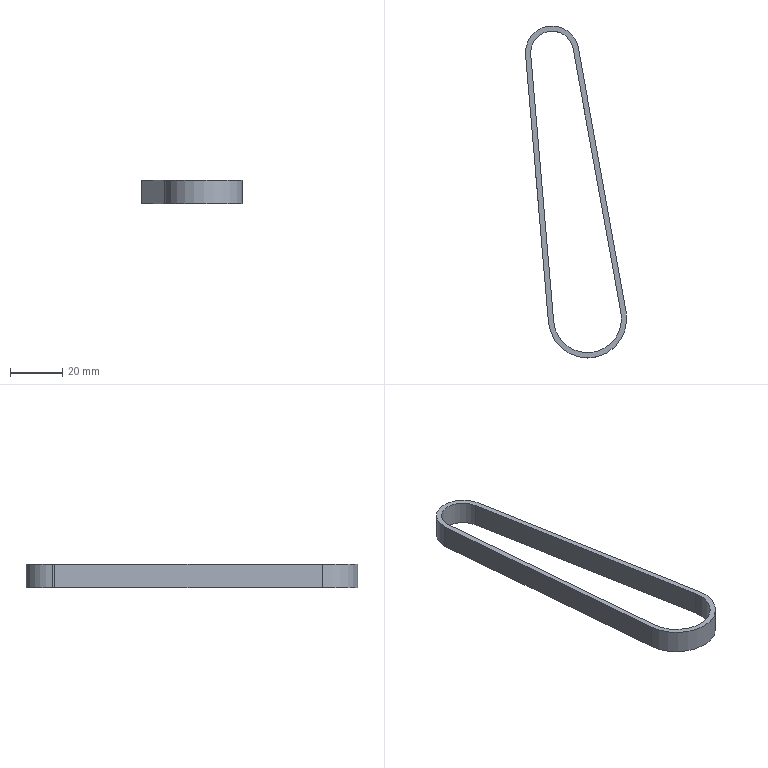Part | NX | features BREP 1 | 1 solid | 12 faces | box 38.615 x 126.615 x 9 mm | volume 4997 mm3 | plane 6 | cylinder 6 | commonest cylinder face diameters 16.34 x2 20.34 x2 25.89 x1 29.89 x1
STEP:
#1=CARTESIAN_POINT('',(26.238,-99.197,-4.5));
#2=VERTEX_POINT('',#1);
#3=CARTESIAN_POINT('',(8.04,1.454,-4.5));
#4=VERTEX_POINT('',#3);
#5=CARTESIAN_POINT('',(8.04,1.454,-4.5));
#6=DIRECTION('',(-0.1779,0.984,0.));
#7=VECTOR('',#6,1000.);
#8=LINE('',#5,#7);
#9=EDGE_CURVE('',#2,#4,#8,.T.);
#10=ORIENTED_EDGE('',*,*,#9,.F.);
#11=CARTESIAN_POINT('',(26.238,-99.197,4.5));
#12=VERTEX_POINT('',#11);
#13=CARTESIAN_POINT('',(26.238,-99.197,4.5));
#14=DIRECTION('',(0.,0.,-1.));
#15=VECTOR('',#14,1000.);
#16=LINE('',#13,#15);
#17=EDGE_CURVE('',#12,#2,#16,.T.);
#18=ORIENTED_EDGE('',*,*,#17,.F.);
#19=CARTESIAN_POINT('',(8.04,1.454,4.5));
#20=VERTEX_POINT('',#19);
#21=CARTESIAN_POINT('',(8.04,1.454,4.5));
#22=DIRECTION('',(-0.1779,0.984,0.));
#23=VECTOR('',#22,1000.);
#24=LINE('',#21,#23);
#25=EDGE_CURVE('',#12,#20,#24,.T.);
#26=ORIENTED_EDGE('',*,*,#25,.T.);
#27=CARTESIAN_POINT('',(8.04,1.454,4.5));
#28=DIRECTION('',(0.,0.,-1.));
#29=VECTOR('',#28,1000.);
#30=LINE('',#27,#29);
#31=EDGE_CURVE('',#20,#4,#30,.T.);
#32=ORIENTED_EDGE('',*,*,#31,.T.);
#33=EDGE_LOOP('',(#10,#18,#26,#32));
#34=FACE_BOUND('',#33,.T.);
#35=CARTESIAN_POINT('',(8.04,1.454,4.5));
#36=DIRECTION('',(-0.984,-0.1779,0.));
#37=DIRECTION('',(0.1779,-0.984,0.));
#38=AXIS2_PLACEMENT_3D('',#35,#36,#37);
#39=PLANE('',#38);
#40=ADVANCED_FACE('',(#34),#39,.T.);
#41=CARTESIAN_POINT('',(0.6024,-102.606,-4.5));
#42=VERTEX_POINT('',#41);
#43=CARTESIAN_POINT('',(13.5,-101.5,-4.5));
#44=DIRECTION('',(0.,0.,1.));
#45=DIRECTION('',(-1.,0.,0.));
#46=AXIS2_PLACEMENT_3D('',#43,#44,#45);
#47=CIRCLE('',#46,12.945);
#48=EDGE_CURVE('',#42,#2,#47,.T.);
#49=ORIENTED_EDGE('',*,*,#48,.F.);
#50=CARTESIAN_POINT('',(0.6024,-102.606,4.5));
#51=VERTEX_POINT('',#50);
#52=CARTESIAN_POINT('',(0.6024,-102.606,4.5));
#53=DIRECTION('',(0.,0.,-1.));
#54=VECTOR('',#53,1000.);
#55=LINE('',#52,#54);
#56=EDGE_CURVE('',#51,#42,#55,.T.);
#57=ORIENTED_EDGE('',*,*,#56,.F.);
#58=CARTESIAN_POINT('',(13.5,-101.5,4.5));
#59=DIRECTION('',(0.,0.,1.));
#60=DIRECTION('',(-1.,0.,0.));
#61=AXIS2_PLACEMENT_3D('',#58,#59,#60);
#62=CIRCLE('',#61,12.945);
#63=EDGE_CURVE('',#51,#12,#62,.T.);
#64=ORIENTED_EDGE('',*,*,#63,.T.);
#65=ORIENTED_EDGE('',*,*,#17,.T.);
#66=EDGE_LOOP('',(#49,#57,#64,#65));
#67=FACE_BOUND('',#66,.T.);
#68=CARTESIAN_POINT('',(13.5,-101.5,4.5));
#69=DIRECTION('',(0.,0.,-1.));
#70=DIRECTION('',(-1.,0.,0.));
#71=AXIS2_PLACEMENT_3D('',#68,#69,#70);
#72=CYLINDRICAL_SURFACE('',#71,12.945);
#73=ADVANCED_FACE('',(#67),#72,.F.);
#74=CARTESIAN_POINT('',(-8.14,-0.6983,-4.5));
#75=VERTEX_POINT('',#74);
#76=CARTESIAN_POINT('',(-8.14,-0.6983,-4.5));
#77=DIRECTION('',(0.08547,-0.9963,0.));
#78=VECTOR('',#77,1000.);
#79=LINE('',#76,#78);
#80=EDGE_CURVE('',#75,#42,#79,.T.);
#81=ORIENTED_EDGE('',*,*,#80,.F.);
#82=CARTESIAN_POINT('',(-8.14,-0.6983,4.5));
#83=VERTEX_POINT('',#82);
#84=CARTESIAN_POINT('',(-8.14,-0.6983,4.5));
#85=DIRECTION('',(0.,0.,-1.));
#86=VECTOR('',#85,1000.);
#87=LINE('',#84,#86);
#88=EDGE_CURVE('',#83,#75,#87,.T.);
#89=ORIENTED_EDGE('',*,*,#88,.F.);
#90=CARTESIAN_POINT('',(-8.14,-0.6983,4.5));
#91=DIRECTION('',(0.08547,-0.9963,0.));
#92=VECTOR('',#91,1000.);
#93=LINE('',#90,#92);
#94=EDGE_CURVE('',#83,#51,#93,.T.);
#95=ORIENTED_EDGE('',*,*,#94,.T.);
#96=ORIENTED_EDGE('',*,*,#56,.T.);
#97=EDGE_LOOP('',(#81,#89,#95,#96));
#98=FACE_BOUND('',#97,.T.);
#99=CARTESIAN_POINT('',(-8.14,-0.6983,4.5));
#100=DIRECTION('',(0.9963,0.08547,0.));
#101=DIRECTION('',(-0.08547,0.9963,0.));
#102=AXIS2_PLACEMENT_3D('',#99,#100,#101);
#103=PLANE('',#102);
#104=ADVANCED_FACE('',(#98),#103,.T.);
#105=CARTESIAN_POINT('',(-8.17,0.,4.5));
#106=VERTEX_POINT('',#105);
#107=CARTESIAN_POINT('',(-8.17,0.,-4.5));
#108=VERTEX_POINT('',#107);
#109=CARTESIAN_POINT('',(-8.17,0.,4.5));
#110=DIRECTION('',(0.,0.,-1.));
#111=VECTOR('',#110,1000.);
#112=LINE('',#109,#111);
#113=EDGE_CURVE('',#106,#108,#112,.T.);
#114=ORIENTED_EDGE('',*,*,#113,.F.);
#115=CARTESIAN_POINT('',(0.,0.,4.5));
#116=DIRECTION('',(0.,0.,1.));
#117=DIRECTION('',(-1.,0.,0.));
#118=AXIS2_PLACEMENT_3D('',#115,#116,#117);
#119=CIRCLE('',#118,8.17);
#120=EDGE_CURVE('',#106,#83,#119,.T.);
#121=ORIENTED_EDGE('',*,*,#120,.T.);
#122=ORIENTED_EDGE('',*,*,#88,.T.);
#123=CARTESIAN_POINT('',(0.,0.,-4.5));
#124=DIRECTION('',(0.,0.,1.));
#125=DIRECTION('',(-1.,0.,0.));
#126=AXIS2_PLACEMENT_3D('',#123,#124,#125);
#127=CIRCLE('',#126,8.17);
#128=EDGE_CURVE('',#108,#75,#127,.T.);
#129=ORIENTED_EDGE('',*,*,#128,.F.);
#130=EDGE_LOOP('',(#114,#121,#122,#129));
#131=FACE_BOUND('',#130,.T.);
#132=CARTESIAN_POINT('',(0.,0.,4.5));
#133=DIRECTION('',(0.,0.,-1.));
#134=DIRECTION('',(-1.,0.,0.));
#135=AXIS2_PLACEMENT_3D('',#132,#133,#134);
#136=CYLINDRICAL_SURFACE('',#135,8.17);
#137=ADVANCED_FACE('',(#131),#136,.F.);
#138=CARTESIAN_POINT('',(28.207,-98.841,-4.5));
#139=VERTEX_POINT('',#138);
#140=CARTESIAN_POINT('',(10.008,1.81,-4.5));
#141=VERTEX_POINT('',#140);
#142=CARTESIAN_POINT('',(10.008,1.81,-4.5));
#143=DIRECTION('',(-0.1779,0.984,0.));
#144=VECTOR('',#143,1000.);
#145=LINE('',#142,#144);
#146=EDGE_CURVE('',#139,#141,#145,.T.);
#147=ORIENTED_EDGE('',*,*,#146,.T.);
#148=CARTESIAN_POINT('',(10.008,1.81,4.5));
#149=VERTEX_POINT('',#148);
#150=CARTESIAN_POINT('',(10.008,1.81,4.5));
#151=DIRECTION('',(0.,0.,-1.));
#152=VECTOR('',#151,1000.);
#153=LINE('',#150,#152);
#154=EDGE_CURVE('',#149,#141,#153,.T.);
#155=ORIENTED_EDGE('',*,*,#154,.F.);
#156=CARTESIAN_POINT('',(28.207,-98.841,4.5));
#157=VERTEX_POINT('',#156);
#158=CARTESIAN_POINT('',(10.008,1.81,4.5));
#159=DIRECTION('',(-0.1779,0.984,0.));
#160=VECTOR('',#159,1000.);
#161=LINE('',#158,#160);
#162=EDGE_CURVE('',#157,#149,#161,.T.);
#163=ORIENTED_EDGE('',*,*,#162,.F.);
#164=CARTESIAN_POINT('',(28.207,-98.841,4.5));
#165=DIRECTION('',(0.,0.,-1.));
#166=VECTOR('',#165,1000.);
#167=LINE('',#164,#166);
#168=EDGE_CURVE('',#157,#139,#167,.T.);
#169=ORIENTED_EDGE('',*,*,#168,.T.);
#170=EDGE_LOOP('',(#147,#155,#163,#169));
#171=FACE_BOUND('',#170,.T.);
#172=CARTESIAN_POINT('',(10.008,1.81,4.5));
#173=DIRECTION('',(-0.984,-0.1779,0.));
#174=DIRECTION('',(0.1779,-0.984,0.));
#175=AXIS2_PLACEMENT_3D('',#172,#173,#174);
#176=PLANE('',#175);
#177=ADVANCED_FACE('',(#171),#176,.F.);
#178=CARTESIAN_POINT('',(-1.39,-102.777,-4.5));
#179=VERTEX_POINT('',#178);
#180=CARTESIAN_POINT('',(13.5,-101.5,-4.5));
#181=DIRECTION('',(0.,0.,1.));
#182=DIRECTION('',(-1.,0.,0.));
#183=AXIS2_PLACEMENT_3D('',#180,#181,#182);
#184=CIRCLE('',#183,14.945);
#185=EDGE_CURVE('',#179,#139,#184,.T.);
#186=ORIENTED_EDGE('',*,*,#185,.T.);
#187=ORIENTED_EDGE('',*,*,#168,.F.);
#188=CARTESIAN_POINT('',(-1.39,-102.777,4.5));
#189=VERTEX_POINT('',#188);
#190=CARTESIAN_POINT('',(13.5,-101.5,4.5));
#191=DIRECTION('',(0.,0.,1.));
#192=DIRECTION('',(-1.,0.,0.));
#193=AXIS2_PLACEMENT_3D('',#190,#191,#192);
#194=CIRCLE('',#193,14.945);
#195=EDGE_CURVE('',#189,#157,#194,.T.);
#196=ORIENTED_EDGE('',*,*,#195,.F.);
#197=CARTESIAN_POINT('',(-1.39,-102.777,4.5));
#198=DIRECTION('',(0.,0.,-1.));
#199=VECTOR('',#198,1000.);
#200=LINE('',#197,#199);
#201=EDGE_CURVE('',#189,#179,#200,.T.);
#202=ORIENTED_EDGE('',*,*,#201,.T.);
#203=EDGE_LOOP('',(#186,#187,#196,#202));
#204=FACE_BOUND('',#203,.T.);
#205=CARTESIAN_POINT('',(13.5,-101.5,4.5));
#206=DIRECTION('',(0.,0.,-1.));
#207=DIRECTION('',(-1.,0.,0.));
#208=AXIS2_PLACEMENT_3D('',#205,#206,#207);
#209=CYLINDRICAL_SURFACE('',#208,14.945);
#210=ADVANCED_FACE('',(#204),#209,.T.);
#211=CARTESIAN_POINT('',(-10.133,-0.8693,-4.5));
#212=VERTEX_POINT('',#211);
#213=CARTESIAN_POINT('',(-10.133,-0.8693,-4.5));
#214=DIRECTION('',(0.08547,-0.9963,0.));
#215=VECTOR('',#214,1000.);
#216=LINE('',#213,#215);
#217=EDGE_CURVE('',#212,#179,#216,.T.);
#218=ORIENTED_EDGE('',*,*,#217,.T.);
#219=ORIENTED_EDGE('',*,*,#201,.F.);
#220=CARTESIAN_POINT('',(-10.133,-0.8693,4.5));
#221=VERTEX_POINT('',#220);
#222=CARTESIAN_POINT('',(-10.133,-0.8693,4.5));
#223=DIRECTION('',(0.08547,-0.9963,0.));
#224=VECTOR('',#223,1000.);
#225=LINE('',#222,#224);
#226=EDGE_CURVE('',#221,#189,#225,.T.);
#227=ORIENTED_EDGE('',*,*,#226,.F.);
#228=CARTESIAN_POINT('',(-10.133,-0.8693,4.5));
#229=DIRECTION('',(0.,0.,-1.));
#230=VECTOR('',#229,1000.);
#231=LINE('',#228,#230);
#232=EDGE_CURVE('',#221,#212,#231,.T.);
#233=ORIENTED_EDGE('',*,*,#232,.T.);
#234=EDGE_LOOP('',(#218,#219,#227,#233));
#235=FACE_BOUND('',#234,.T.);
#236=CARTESIAN_POINT('',(-10.133,-0.8693,4.5));
#237=DIRECTION('',(0.9963,0.08547,0.));
#238=DIRECTION('',(-0.08547,0.9963,0.));
#239=AXIS2_PLACEMENT_3D('',#236,#237,#238);
#240=PLANE('',#239);
#241=ADVANCED_FACE('',(#235),#240,.F.);
#242=CARTESIAN_POINT('',(-10.17,0.,4.5));
#243=VERTEX_POINT('',#242);
#244=CARTESIAN_POINT('',(-10.17,0.,-4.5));
#245=VERTEX_POINT('',#244);
#246=CARTESIAN_POINT('',(-10.17,0.,4.5));
#247=DIRECTION('',(0.,0.,-1.));
#248=VECTOR('',#247,1000.);
#249=LINE('',#246,#248);
#250=EDGE_CURVE('',#243,#245,#249,.T.);
#251=ORIENTED_EDGE('',*,*,#250,.F.);
#252=CARTESIAN_POINT('',(0.,0.,4.5));
#253=DIRECTION('',(0.,0.,1.));
#254=DIRECTION('',(-1.,0.,0.));
#255=AXIS2_PLACEMENT_3D('',#252,#253,#254);
#256=CIRCLE('',#255,10.17);
#257=EDGE_CURVE('',#149,#243,#256,.T.);
#258=ORIENTED_EDGE('',*,*,#257,.F.);
#259=ORIENTED_EDGE('',*,*,#154,.T.);
#260=CARTESIAN_POINT('',(0.,0.,-4.5));
#261=DIRECTION('',(0.,0.,1.));
#262=DIRECTION('',(-1.,0.,0.));
#263=AXIS2_PLACEMENT_3D('',#260,#261,#262);
#264=CIRCLE('',#263,10.17);
#265=EDGE_CURVE('',#141,#245,#264,.T.);
#266=ORIENTED_EDGE('',*,*,#265,.T.);
#267=EDGE_LOOP('',(#251,#258,#259,#266));
#268=FACE_BOUND('',#267,.T.);
#269=CARTESIAN_POINT('',(0.,0.,4.5));
#270=DIRECTION('',(0.,0.,-1.));
#271=DIRECTION('',(-1.,0.,0.));
#272=AXIS2_PLACEMENT_3D('',#269,#270,#271);
#273=CYLINDRICAL_SURFACE('',#272,10.17);
#274=ADVANCED_FACE('',(#268),#273,.T.);
#275=ORIENTED_EDGE('',*,*,#9,.T.);
#276=CARTESIAN_POINT('',(0.,0.,-4.5));
#277=DIRECTION('',(0.,0.,1.));
#278=DIRECTION('',(-1.,0.,0.));
#279=AXIS2_PLACEMENT_3D('',#276,#277,#278);
#280=CIRCLE('',#279,8.17);
#281=EDGE_CURVE('',#4,#108,#280,.T.);
#282=ORIENTED_EDGE('',*,*,#281,.T.);
#283=ORIENTED_EDGE('',*,*,#128,.T.);
#284=ORIENTED_EDGE('',*,*,#80,.T.);
#285=ORIENTED_EDGE('',*,*,#48,.T.);
#286=EDGE_LOOP('',(#275,#282,#283,#284,#285));
#287=FACE_BOUND('',#286,.T.);
#288=ORIENTED_EDGE('',*,*,#265,.F.);
#289=ORIENTED_EDGE('',*,*,#146,.F.);
#290=ORIENTED_EDGE('',*,*,#185,.F.);
#291=ORIENTED_EDGE('',*,*,#217,.F.);
#292=CARTESIAN_POINT('',(0.,0.,-4.5));
#293=DIRECTION('',(0.,0.,1.));
#294=DIRECTION('',(-1.,0.,0.));
#295=AXIS2_PLACEMENT_3D('',#292,#293,#294);
#296=CIRCLE('',#295,10.17);
#297=EDGE_CURVE('',#245,#212,#296,.T.);
#298=ORIENTED_EDGE('',*,*,#297,.F.);
#299=EDGE_LOOP('',(#288,#289,#290,#291,#298));
#300=FACE_BOUND('',#299,.T.);
#301=CARTESIAN_POINT('',(0.,0.,-4.5));
#302=DIRECTION('',(0.,0.,-1.));
#303=DIRECTION('',(-1.,0.,0.));
#304=AXIS2_PLACEMENT_3D('',#301,#302,#303);
#305=PLANE('',#304);
#306=ADVANCED_FACE('',(#287,#300),#305,.T.);
#307=CARTESIAN_POINT('',(0.,0.,4.5));
#308=DIRECTION('',(0.,0.,1.));
#309=DIRECTION('',(-1.,0.,0.));
#310=AXIS2_PLACEMENT_3D('',#307,#308,#309);
#311=CIRCLE('',#310,8.17);
#312=EDGE_CURVE('',#20,#106,#311,.T.);
#313=ORIENTED_EDGE('',*,*,#312,.F.);
#314=ORIENTED_EDGE('',*,*,#25,.F.);
#315=ORIENTED_EDGE('',*,*,#63,.F.);
#316=ORIENTED_EDGE('',*,*,#94,.F.);
#317=ORIENTED_EDGE('',*,*,#120,.F.);
#318=EDGE_LOOP('',(#313,#314,#315,#316,#317));
#319=FACE_BOUND('',#318,.T.);
#320=ORIENTED_EDGE('',*,*,#257,.T.);
#321=CARTESIAN_POINT('',(0.,0.,4.5));
#322=DIRECTION('',(0.,0.,1.));
#323=DIRECTION('',(-1.,0.,0.));
#324=AXIS2_PLACEMENT_3D('',#321,#322,#323);
#325=CIRCLE('',#324,10.17);
#326=EDGE_CURVE('',#243,#221,#325,.T.);
#327=ORIENTED_EDGE('',*,*,#326,.T.);
#328=ORIENTED_EDGE('',*,*,#226,.T.);
#329=ORIENTED_EDGE('',*,*,#195,.T.);
#330=ORIENTED_EDGE('',*,*,#162,.T.);
#331=EDGE_LOOP('',(#320,#327,#328,#329,#330));
#332=FACE_BOUND('',#331,.T.);
#333=CARTESIAN_POINT('',(0.,0.,4.5));
#334=DIRECTION('',(0.,0.,-1.));
#335=DIRECTION('',(-1.,0.,0.));
#336=AXIS2_PLACEMENT_3D('',#333,#334,#335);
#337=PLANE('',#336);
#338=ADVANCED_FACE('',(#319,#332),#337,.F.);
#339=ORIENTED_EDGE('',*,*,#326,.F.);
#340=ORIENTED_EDGE('',*,*,#250,.T.);
#341=ORIENTED_EDGE('',*,*,#297,.T.);
#342=ORIENTED_EDGE('',*,*,#232,.F.);
#343=EDGE_LOOP('',(#339,#340,#341,#342));
#344=FACE_BOUND('',#343,.T.);
#345=CARTESIAN_POINT('',(0.,0.,4.5));
#346=DIRECTION('',(0.,0.,-1.));
#347=DIRECTION('',(-1.,0.,0.));
#348=AXIS2_PLACEMENT_3D('',#345,#346,#347);
#349=CYLINDRICAL_SURFACE('',#348,10.17);
#350=ADVANCED_FACE('',(#344),#349,.T.);
#351=ORIENTED_EDGE('',*,*,#312,.T.);
#352=ORIENTED_EDGE('',*,*,#113,.T.);
#353=ORIENTED_EDGE('',*,*,#281,.F.);
#354=ORIENTED_EDGE('',*,*,#31,.F.);
#355=EDGE_LOOP('',(#351,#352,#353,#354));
#356=FACE_BOUND('',#355,.T.);
#357=CARTESIAN_POINT('',(0.,0.,4.5));
#358=DIRECTION('',(0.,0.,-1.));
#359=DIRECTION('',(-1.,0.,0.));
#360=AXIS2_PLACEMENT_3D('',#357,#358,#359);
#361=CYLINDRICAL_SURFACE('',#360,8.17);
#362=ADVANCED_FACE('',(#356),#361,.F.);
#363=CLOSED_SHELL('',(#40,#73,#104,#137,#177,#210,#241,#274,#306,#338,#350,#362));
#364=MANIFOLD_SOLID_BREP('',#363);
#365=(LENGTH_UNIT()NAMED_UNIT(*)SI_UNIT(.MILLI.,.METRE.));
#366=UNCERTAINTY_MEASURE_WITH_UNIT(LENGTH_MEASURE(0.00001),#365,'','');
#367=(NAMED_UNIT(*)PLANE_ANGLE_UNIT()SI_UNIT($,.RADIAN.));
#368=(NAMED_UNIT(*)SI_UNIT($,.STERADIAN.)SOLID_ANGLE_UNIT());
#369=(GEOMETRIC_REPRESENTATION_CONTEXT(3)GLOBAL_UNCERTAINTY_ASSIGNED_CONTEXT((#366))GLOBAL_UNIT_ASSIGNED_CONTEXT((#365,#367,#368))REPRESENTATION_CONTEXT('',''));
#370=ADVANCED_BREP_SHAPE_REPRESENTATION('',(#364),#369);